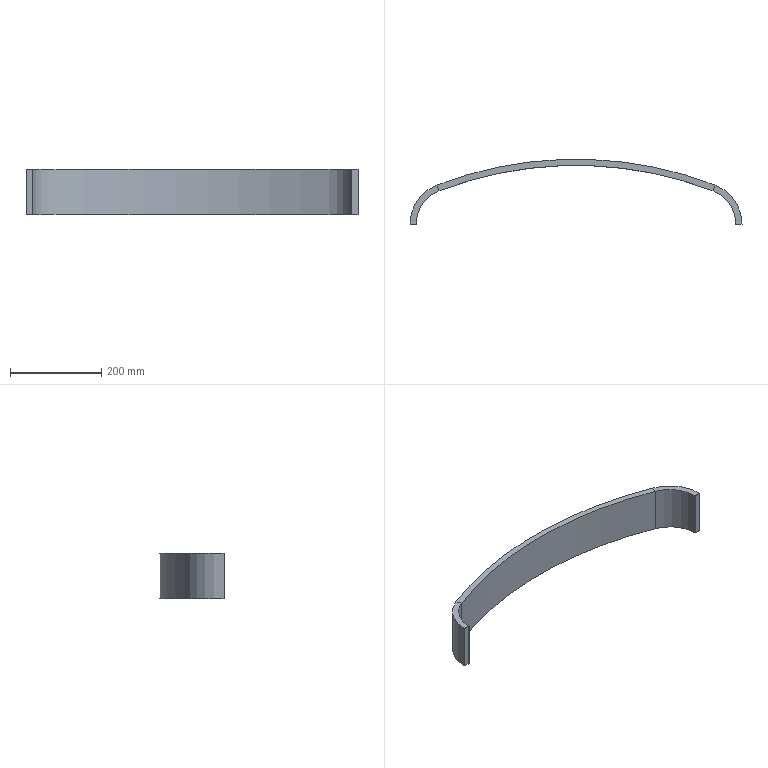Part | SolidWorks | features FlatPattern 1, HoleWzd 1, ICE 1, SMBaseFlange 1, SheetMetal 1 | 1 solid | 22 faces | box 727 x 142.5 x 100 mm | volume 1111821 mm3 | plane 16 | cylinder 6 | commonest cylinder face diameters 156.075 x2 183.075 x2 1670 x1 1697 x1
STEP:
#1=CARTESIAN_POINT('',(50.,0.4197,100.));
#2=VERTEX_POINT('',#1);
#3=CARTESIAN_POINT('',(36.5,0.4197,100.));
#4=VERTEX_POINT('',#3);
#5=CARTESIAN_POINT('',(50.,0.4197,100.));
#6=DIRECTION('',(-1.,0.,0.));
#7=VECTOR('',#6,1000.);
#8=LINE('',#5,#7);
#9=EDGE_CURVE('',#2,#4,#8,.T.);
#10=ORIENTED_EDGE('',*,*,#9,.F.);
#11=CARTESIAN_POINT('',(100.,73.246,100.));
#12=VERTEX_POINT('',#11);
#13=CARTESIAN_POINT('',(128.037,0.4197,100.));
#14=DIRECTION('',(0.,0.,1.));
#15=DIRECTION('',(1.,0.,0.));
#16=AXIS2_PLACEMENT_3D('',#13,#14,#15);
#17=CIRCLE('',#16,78.037);
#18=EDGE_CURVE('',#12,#2,#17,.T.);
#19=ORIENTED_EDGE('',*,*,#18,.F.);
#20=CARTESIAN_POINT('',(95.15,85.845,100.));
#21=VERTEX_POINT('',#20);
#22=CARTESIAN_POINT('',(100.,73.246,100.));
#23=DIRECTION('',(-0.3593,0.9332,0.));
#24=VECTOR('',#23,1000.);
#25=LINE('',#22,#24);
#26=EDGE_CURVE('',#12,#21,#25,.T.);
#27=ORIENTED_EDGE('',*,*,#26,.T.);
#28=CARTESIAN_POINT('',(128.037,0.4197,100.));
#29=DIRECTION('',(0.,0.,1.));
#30=DIRECTION('',(1.,0.,0.));
#31=AXIS2_PLACEMENT_3D('',#28,#29,#30);
#32=CIRCLE('',#31,91.537);
#33=EDGE_CURVE('',#21,#4,#32,.T.);
#34=ORIENTED_EDGE('',*,*,#33,.T.);
#35=EDGE_LOOP('',(#10,#19,#27,#34));
#36=FACE_OUTER_BOUND('',#35,.T.);
#37=CARTESIAN_POINT('',(50.,0.4197,100.));
#38=DIRECTION('',(0.,0.,1.));
#39=DIRECTION('',(1.,0.,0.));
#40=AXIS2_PLACEMENT_3D('',#37,#38,#39);
#41=PLANE('',#40);
#42=ADVANCED_FACE('',(#36),#41,.T.);
#43=CARTESIAN_POINT('',(36.5,0.4197,0.));
#44=VERTEX_POINT('',#43);
#45=CARTESIAN_POINT('',(50.,0.4197,0.));
#46=VERTEX_POINT('',#45);
#47=CARTESIAN_POINT('',(36.5,0.4197,0.));
#48=DIRECTION('',(1.,0.,0.));
#49=VECTOR('',#48,1000.);
#50=LINE('',#47,#49);
#51=EDGE_CURVE('',#44,#46,#50,.T.);
#52=ORIENTED_EDGE('',*,*,#51,.F.);
#53=CARTESIAN_POINT('',(95.15,85.845,0.));
#54=VERTEX_POINT('',#53);
#55=CARTESIAN_POINT('',(128.037,0.4197,0.));
#56=DIRECTION('',(0.,0.,1.));
#57=DIRECTION('',(1.,0.,0.));
#58=AXIS2_PLACEMENT_3D('',#55,#56,#57);
#59=CIRCLE('',#58,91.537);
#60=EDGE_CURVE('',#54,#44,#59,.T.);
#61=ORIENTED_EDGE('',*,*,#60,.F.);
#62=CARTESIAN_POINT('',(100.,73.246,0.));
#63=VERTEX_POINT('',#62);
#64=CARTESIAN_POINT('',(95.15,85.845,0.));
#65=DIRECTION('',(0.3593,-0.9332,0.));
#66=VECTOR('',#65,1000.);
#67=LINE('',#64,#66);
#68=EDGE_CURVE('',#54,#63,#67,.T.);
#69=ORIENTED_EDGE('',*,*,#68,.T.);
#70=CARTESIAN_POINT('',(128.037,0.4197,0.));
#71=DIRECTION('',(0.,0.,1.));
#72=DIRECTION('',(1.,0.,0.));
#73=AXIS2_PLACEMENT_3D('',#70,#71,#72);
#74=CIRCLE('',#73,78.037);
#75=EDGE_CURVE('',#63,#46,#74,.T.);
#76=ORIENTED_EDGE('',*,*,#75,.T.);
#77=EDGE_LOOP('',(#52,#61,#69,#76));
#78=FACE_OUTER_BOUND('',#77,.T.);
#79=CARTESIAN_POINT('',(36.5,0.4197,0.));
#80=DIRECTION('',(0.,0.,-1.));
#81=DIRECTION('',(-1.,0.,0.));
#82=AXIS2_PLACEMENT_3D('',#79,#80,#81);
#83=PLANE('',#82);
#84=ADVANCED_FACE('',(#78),#83,.T.);
#85=ORIENTED_EDGE('',*,*,#26,.F.);
#86=CARTESIAN_POINT('',(700.,73.246,100.));
#87=VERTEX_POINT('',#86);
#88=CARTESIAN_POINT('',(400.,-706.,100.));
#89=DIRECTION('',(0.,0.,1.));
#90=DIRECTION('',(-1.,0.,0.));
#91=AXIS2_PLACEMENT_3D('',#88,#89,#90);
#92=CIRCLE('',#91,835.);
#93=EDGE_CURVE('',#87,#12,#92,.T.);
#94=ORIENTED_EDGE('',*,*,#93,.F.);
#95=CARTESIAN_POINT('',(704.85,85.845,100.));
#96=VERTEX_POINT('',#95);
#97=CARTESIAN_POINT('',(700.,73.246,100.));
#98=DIRECTION('',(0.3593,0.9332,0.));
#99=VECTOR('',#98,1000.);
#100=LINE('',#97,#99);
#101=EDGE_CURVE('',#87,#96,#100,.T.);
#102=ORIENTED_EDGE('',*,*,#101,.T.);
#103=CARTESIAN_POINT('',(400.,-706.,100.));
#104=DIRECTION('',(0.,0.,1.));
#105=DIRECTION('',(1.,0.,0.));
#106=AXIS2_PLACEMENT_3D('',#103,#104,#105);
#107=CIRCLE('',#106,848.5);
#108=EDGE_CURVE('',#96,#21,#107,.T.);
#109=ORIENTED_EDGE('',*,*,#108,.T.);
#110=EDGE_LOOP('',(#85,#94,#102,#109));
#111=FACE_OUTER_BOUND('',#110,.T.);
#112=CARTESIAN_POINT('',(100.,73.246,100.));
#113=DIRECTION('',(0.,0.,1.));
#114=DIRECTION('',(1.,0.,0.));
#115=AXIS2_PLACEMENT_3D('',#112,#113,#114);
#116=PLANE('',#115);
#117=ADVANCED_FACE('',(#111),#116,.T.);
#118=ORIENTED_EDGE('',*,*,#68,.F.);
#119=CARTESIAN_POINT('',(704.85,85.845,0.));
#120=VERTEX_POINT('',#119);
#121=CARTESIAN_POINT('',(400.,-706.,0.));
#122=DIRECTION('',(0.,0.,1.));
#123=DIRECTION('',(1.,0.,0.));
#124=AXIS2_PLACEMENT_3D('',#121,#122,#123);
#125=CIRCLE('',#124,848.5);
#126=EDGE_CURVE('',#120,#54,#125,.T.);
#127=ORIENTED_EDGE('',*,*,#126,.F.);
#128=CARTESIAN_POINT('',(700.,73.246,0.));
#129=VERTEX_POINT('',#128);
#130=CARTESIAN_POINT('',(704.85,85.845,0.));
#131=DIRECTION('',(-0.3593,-0.9332,0.));
#132=VECTOR('',#131,1000.);
#133=LINE('',#130,#132);
#134=EDGE_CURVE('',#120,#129,#133,.T.);
#135=ORIENTED_EDGE('',*,*,#134,.T.);
#136=CARTESIAN_POINT('',(400.,-706.,0.));
#137=DIRECTION('',(0.,0.,1.));
#138=DIRECTION('',(-1.,0.,0.));
#139=AXIS2_PLACEMENT_3D('',#136,#137,#138);
#140=CIRCLE('',#139,835.);
#141=EDGE_CURVE('',#129,#63,#140,.T.);
#142=ORIENTED_EDGE('',*,*,#141,.T.);
#143=EDGE_LOOP('',(#118,#127,#135,#142));
#144=FACE_OUTER_BOUND('',#143,.T.);
#145=CARTESIAN_POINT('',(95.15,85.845,0.));
#146=DIRECTION('',(0.,0.,-1.));
#147=DIRECTION('',(-1.,0.,0.));
#148=AXIS2_PLACEMENT_3D('',#145,#146,#147);
#149=PLANE('',#148);
#150=ADVANCED_FACE('',(#144),#149,.T.);
#151=ORIENTED_EDGE('',*,*,#101,.F.);
#152=CARTESIAN_POINT('',(750.,0.4197,100.));
#153=VERTEX_POINT('',#152);
#154=CARTESIAN_POINT('',(671.963,0.4197,100.));
#155=DIRECTION('',(0.,0.,1.));
#156=DIRECTION('',(-1.,0.,0.));
#157=AXIS2_PLACEMENT_3D('',#154,#155,#156);
#158=CIRCLE('',#157,78.037);
#159=EDGE_CURVE('',#153,#87,#158,.T.);
#160=ORIENTED_EDGE('',*,*,#159,.F.);
#161=CARTESIAN_POINT('',(763.5,0.4197,100.));
#162=VERTEX_POINT('',#161);
#163=CARTESIAN_POINT('',(763.5,0.4197,100.));
#164=DIRECTION('',(-1.,0.,0.));
#165=VECTOR('',#164,1000.);
#166=LINE('',#163,#165);
#167=EDGE_CURVE('',#162,#153,#166,.T.);
#168=ORIENTED_EDGE('',*,*,#167,.F.);
#169=CARTESIAN_POINT('',(671.963,0.4197,100.));
#170=DIRECTION('',(0.,0.,1.));
#171=DIRECTION('',(1.,0.,0.));
#172=AXIS2_PLACEMENT_3D('',#169,#170,#171);
#173=CIRCLE('',#172,91.537);
#174=EDGE_CURVE('',#162,#96,#173,.T.);
#175=ORIENTED_EDGE('',*,*,#174,.T.);
#176=EDGE_LOOP('',(#151,#160,#168,#175));
#177=FACE_OUTER_BOUND('',#176,.T.);
#178=CARTESIAN_POINT('',(700.,73.246,100.));
#179=DIRECTION('',(0.,0.,1.));
#180=DIRECTION('',(1.,0.,0.));
#181=AXIS2_PLACEMENT_3D('',#178,#179,#180);
#182=PLANE('',#181);
#183=ADVANCED_FACE('',(#177),#182,.T.);
#184=CARTESIAN_POINT('',(50.,0.,100.));
#185=VERTEX_POINT('',#184);
#186=CARTESIAN_POINT('',(50.,0.,100.));
#187=DIRECTION('',(0.,-1.,0.));
#188=VECTOR('',#187,1000.);
#189=LINE('',#186,#188);
#190=EDGE_CURVE('',#2,#185,#189,.T.);
#191=ORIENTED_EDGE('',*,*,#190,.F.);
#192=ORIENTED_EDGE('',*,*,#9,.T.);
#193=CARTESIAN_POINT('',(36.5,0.,100.));
#194=VERTEX_POINT('',#193);
#195=CARTESIAN_POINT('',(36.5,0.,100.));
#196=DIRECTION('',(0.,-1.,0.));
#197=VECTOR('',#196,1000.);
#198=LINE('',#195,#197);
#199=EDGE_CURVE('',#4,#194,#198,.T.);
#200=ORIENTED_EDGE('',*,*,#199,.T.);
#201=CARTESIAN_POINT('',(50.,0.,100.));
#202=DIRECTION('',(-1.,0.,0.));
#203=VECTOR('',#202,1000.);
#204=LINE('',#201,#203);
#205=EDGE_CURVE('',#185,#194,#204,.T.);
#206=ORIENTED_EDGE('',*,*,#205,.F.);
#207=EDGE_LOOP('',(#191,#192,#200,#206));
#208=FACE_OUTER_BOUND('',#207,.T.);
#209=CARTESIAN_POINT('',(763.5,0.4197,100.));
#210=DIRECTION('',(0.,0.,1.));
#211=DIRECTION('',(1.,0.,0.));
#212=AXIS2_PLACEMENT_3D('',#209,#210,#211);
#213=PLANE('',#212);
#214=ADVANCED_FACE('',(#208),#213,.T.);
#215=CARTESIAN_POINT('',(750.,0.4197,0.));
#216=VERTEX_POINT('',#215);
#217=CARTESIAN_POINT('',(763.5,0.4197,0.));
#218=VERTEX_POINT('',#217);
#219=CARTESIAN_POINT('',(750.,0.4197,0.));
#220=DIRECTION('',(1.,0.,0.));
#221=VECTOR('',#220,1000.);
#222=LINE('',#219,#221);
#223=EDGE_CURVE('',#216,#218,#222,.T.);
#224=ORIENTED_EDGE('',*,*,#223,.F.);
#225=CARTESIAN_POINT('',(671.963,0.4197,0.));
#226=DIRECTION('',(0.,0.,1.));
#227=DIRECTION('',(-1.,0.,0.));
#228=AXIS2_PLACEMENT_3D('',#225,#226,#227);
#229=CIRCLE('',#228,78.037);
#230=EDGE_CURVE('',#216,#129,#229,.T.);
#231=ORIENTED_EDGE('',*,*,#230,.T.);
#232=ORIENTED_EDGE('',*,*,#134,.F.);
#233=CARTESIAN_POINT('',(671.963,0.4197,0.));
#234=DIRECTION('',(0.,0.,1.));
#235=DIRECTION('',(1.,0.,0.));
#236=AXIS2_PLACEMENT_3D('',#233,#234,#235);
#237=CIRCLE('',#236,91.537);
#238=EDGE_CURVE('',#218,#120,#237,.T.);
#239=ORIENTED_EDGE('',*,*,#238,.F.);
#240=EDGE_LOOP('',(#224,#231,#232,#239));
#241=FACE_OUTER_BOUND('',#240,.T.);
#242=CARTESIAN_POINT('',(750.,0.4197,0.));
#243=DIRECTION('',(0.,0.,-1.));
#244=DIRECTION('',(-1.,0.,0.));
#245=AXIS2_PLACEMENT_3D('',#242,#243,#244);
#246=PLANE('',#245);
#247=ADVANCED_FACE('',(#241),#246,.T.);
#248=CARTESIAN_POINT('',(750.,0.,0.));
#249=VERTEX_POINT('',#248);
#250=CARTESIAN_POINT('',(750.,0.,0.));
#251=DIRECTION('',(0.,1.,0.));
#252=VECTOR('',#251,1000.);
#253=LINE('',#250,#252);
#254=EDGE_CURVE('',#249,#216,#253,.T.);
#255=ORIENTED_EDGE('',*,*,#254,.T.);
#256=ORIENTED_EDGE('',*,*,#223,.T.);
#257=CARTESIAN_POINT('',(763.5,0.,0.));
#258=VERTEX_POINT('',#257);
#259=CARTESIAN_POINT('',(763.5,0.,0.));
#260=DIRECTION('',(0.,1.,0.));
#261=VECTOR('',#260,1000.);
#262=LINE('',#259,#261);
#263=EDGE_CURVE('',#258,#218,#262,.T.);
#264=ORIENTED_EDGE('',*,*,#263,.F.);
#265=CARTESIAN_POINT('',(763.5,0.,0.));
#266=DIRECTION('',(-1.,0.,0.));
#267=VECTOR('',#266,1000.);
#268=LINE('',#265,#267);
#269=EDGE_CURVE('',#258,#249,#268,.T.);
#270=ORIENTED_EDGE('',*,*,#269,.T.);
#271=EDGE_LOOP('',(#255,#256,#264,#270));
#272=FACE_OUTER_BOUND('',#271,.T.);
#273=CARTESIAN_POINT('',(704.85,85.845,0.));
#274=DIRECTION('',(0.,0.,-1.));
#275=DIRECTION('',(-1.,0.,0.));
#276=AXIS2_PLACEMENT_3D('',#273,#274,#275);
#277=PLANE('',#276);
#278=ADVANCED_FACE('',(#272),#277,.T.);
#279=CARTESIAN_POINT('',(36.5,0.,0.));
#280=VERTEX_POINT('',#279);
#281=CARTESIAN_POINT('',(36.5,0.,0.));
#282=DIRECTION('',(0.,-1.,0.));
#283=VECTOR('',#282,1000.);
#284=LINE('',#281,#283);
#285=EDGE_CURVE('',#44,#280,#284,.T.);
#286=ORIENTED_EDGE('',*,*,#285,.T.);
#287=CARTESIAN_POINT('',(36.5,0.,100.));
#288=DIRECTION('',(0.,0.,-1.));
#289=VECTOR('',#288,1000.);
#290=LINE('',#287,#289);
#291=EDGE_CURVE('',#194,#280,#290,.T.);
#292=ORIENTED_EDGE('',*,*,#291,.F.);
#293=ORIENTED_EDGE('',*,*,#199,.F.);
#294=CARTESIAN_POINT('',(36.5,0.4197,100.));
#295=DIRECTION('',(0.,0.,-1.));
#296=VECTOR('',#295,1000.);
#297=LINE('',#294,#296);
#298=EDGE_CURVE('',#4,#44,#297,.T.);
#299=ORIENTED_EDGE('',*,*,#298,.T.);
#300=EDGE_LOOP('',(#286,#292,#293,#299));
#301=FACE_OUTER_BOUND('',#300,.T.);
#302=CARTESIAN_POINT('',(36.5,0.,100.));
#303=DIRECTION('',(1.,0.,0.));
#304=DIRECTION('',(0.,1.,0.));
#305=AXIS2_PLACEMENT_3D('',#302,#303,#304);
#306=PLANE('',#305);
#307=ADVANCED_FACE('',(#301),#306,.F.);
#308=CARTESIAN_POINT('',(50.,0.,0.));
#309=VERTEX_POINT('',#308);
#310=CARTESIAN_POINT('',(50.,0.,0.));
#311=DIRECTION('',(-1.,0.,0.));
#312=VECTOR('',#311,1000.);
#313=LINE('',#310,#312);
#314=EDGE_CURVE('',#309,#280,#313,.T.);
#315=ORIENTED_EDGE('',*,*,#314,.F.);
#316=CARTESIAN_POINT('',(50.,0.,100.));
#317=DIRECTION('',(0.,0.,-1.));
#318=VECTOR('',#317,1000.);
#319=LINE('',#316,#318);
#320=EDGE_CURVE('',#185,#309,#319,.T.);
#321=ORIENTED_EDGE('',*,*,#320,.F.);
#322=ORIENTED_EDGE('',*,*,#205,.T.);
#323=ORIENTED_EDGE('',*,*,#291,.T.);
#324=EDGE_LOOP('',(#315,#321,#322,#323));
#325=FACE_OUTER_BOUND('',#324,.T.);
#326=CARTESIAN_POINT('',(50.,0.,100.));
#327=DIRECTION('',(0.,-1.,0.));
#328=DIRECTION('',(1.,0.,0.));
#329=AXIS2_PLACEMENT_3D('',#326,#327,#328);
#330=PLANE('',#329);
#331=ADVANCED_FACE('',(#325),#330,.T.);
#332=CARTESIAN_POINT('',(50.,0.,0.));
#333=DIRECTION('',(0.,-1.,0.));
#334=VECTOR('',#333,1000.);
#335=LINE('',#332,#334);
#336=EDGE_CURVE('',#46,#309,#335,.T.);
#337=ORIENTED_EDGE('',*,*,#336,.F.);
#338=CARTESIAN_POINT('',(50.,0.4197,100.));
#339=DIRECTION('',(0.,0.,-1.));
#340=VECTOR('',#339,1000.);
#341=LINE('',#338,#340);
#342=EDGE_CURVE('',#2,#46,#341,.T.);
#343=ORIENTED_EDGE('',*,*,#342,.F.);
#344=ORIENTED_EDGE('',*,*,#190,.T.);
#345=ORIENTED_EDGE('',*,*,#320,.T.);
#346=EDGE_LOOP('',(#337,#343,#344,#345));
#347=FACE_OUTER_BOUND('',#346,.T.);
#348=CARTESIAN_POINT('',(50.,0.,100.));
#349=DIRECTION('',(1.,0.,0.));
#350=DIRECTION('',(0.,1.,0.));
#351=AXIS2_PLACEMENT_3D('',#348,#349,#350);
#352=PLANE('',#351);
#353=ADVANCED_FACE('',(#347),#352,.T.);
#354=ORIENTED_EDGE('',*,*,#75,.F.);
#355=CARTESIAN_POINT('',(100.,73.246,100.));
#356=DIRECTION('',(0.,0.,-1.));
#357=VECTOR('',#356,1000.);
#358=LINE('',#355,#357);
#359=EDGE_CURVE('',#12,#63,#358,.T.);
#360=ORIENTED_EDGE('',*,*,#359,.F.);
#361=ORIENTED_EDGE('',*,*,#18,.T.);
#362=ORIENTED_EDGE('',*,*,#342,.T.);
#363=EDGE_LOOP('',(#354,#360,#361,#362));
#364=FACE_OUTER_BOUND('',#363,.T.);
#365=CARTESIAN_POINT('',(128.037,0.4197,100.));
#366=DIRECTION('',(0.,0.,-1.));
#367=DIRECTION('',(-1.,0.,0.));
#368=AXIS2_PLACEMENT_3D('',#365,#366,#367);
#369=CYLINDRICAL_SURFACE('',#368,78.037);
#370=ADVANCED_FACE('',(#364),#369,.F.);
#371=ORIENTED_EDGE('',*,*,#141,.F.);
#372=CARTESIAN_POINT('',(700.,73.246,100.));
#373=DIRECTION('',(0.,0.,-1.));
#374=VECTOR('',#373,1000.);
#375=LINE('',#372,#374);
#376=EDGE_CURVE('',#87,#129,#375,.T.);
#377=ORIENTED_EDGE('',*,*,#376,.F.);
#378=ORIENTED_EDGE('',*,*,#93,.T.);
#379=ORIENTED_EDGE('',*,*,#359,.T.);
#380=EDGE_LOOP('',(#371,#377,#378,#379));
#381=FACE_OUTER_BOUND('',#380,.T.);
#382=CARTESIAN_POINT('',(400.,-706.,100.));
#383=DIRECTION('',(0.,0.,-1.));
#384=DIRECTION('',(-1.,0.,0.));
#385=AXIS2_PLACEMENT_3D('',#382,#383,#384);
#386=CYLINDRICAL_SURFACE('',#385,835.);
#387=ADVANCED_FACE('',(#381),#386,.F.);
#388=ORIENTED_EDGE('',*,*,#230,.F.);
#389=CARTESIAN_POINT('',(750.,0.4197,100.));
#390=DIRECTION('',(0.,0.,-1.));
#391=VECTOR('',#390,1000.);
#392=LINE('',#389,#391);
#393=EDGE_CURVE('',#153,#216,#392,.T.);
#394=ORIENTED_EDGE('',*,*,#393,.F.);
#395=ORIENTED_EDGE('',*,*,#159,.T.);
#396=ORIENTED_EDGE('',*,*,#376,.T.);
#397=EDGE_LOOP('',(#388,#394,#395,#396));
#398=FACE_OUTER_BOUND('',#397,.T.);
#399=CARTESIAN_POINT('',(671.963,0.4197,100.));
#400=DIRECTION('',(0.,0.,-1.));
#401=DIRECTION('',(-1.,0.,0.));
#402=AXIS2_PLACEMENT_3D('',#399,#400,#401);
#403=CYLINDRICAL_SURFACE('',#402,78.037);
#404=ADVANCED_FACE('',(#398),#403,.F.);
#405=ORIENTED_EDGE('',*,*,#254,.F.);
#406=CARTESIAN_POINT('',(750.,0.,100.));
#407=VERTEX_POINT('',#406);
#408=CARTESIAN_POINT('',(750.,0.,100.));
#409=DIRECTION('',(0.,0.,-1.));
#410=VECTOR('',#409,1000.);
#411=LINE('',#408,#410);
#412=EDGE_CURVE('',#407,#249,#411,.T.);
#413=ORIENTED_EDGE('',*,*,#412,.F.);
#414=CARTESIAN_POINT('',(750.,0.,100.));
#415=DIRECTION('',(0.,1.,0.));
#416=VECTOR('',#415,1000.);
#417=LINE('',#414,#416);
#418=EDGE_CURVE('',#407,#153,#417,.T.);
#419=ORIENTED_EDGE('',*,*,#418,.T.);
#420=ORIENTED_EDGE('',*,*,#393,.T.);
#421=EDGE_LOOP('',(#405,#413,#419,#420));
#422=FACE_OUTER_BOUND('',#421,.T.);
#423=CARTESIAN_POINT('',(750.,0.,100.));
#424=DIRECTION('',(-1.,0.,0.));
#425=DIRECTION('',(0.,0.,1.));
#426=AXIS2_PLACEMENT_3D('',#423,#424,#425);
#427=PLANE('',#426);
#428=ADVANCED_FACE('',(#422),#427,.T.);
#429=ORIENTED_EDGE('',*,*,#269,.F.);
#430=CARTESIAN_POINT('',(763.5,0.,100.));
#431=VERTEX_POINT('',#430);
#432=CARTESIAN_POINT('',(763.5,0.,100.));
#433=DIRECTION('',(0.,0.,-1.));
#434=VECTOR('',#433,1000.);
#435=LINE('',#432,#434);
#436=EDGE_CURVE('',#431,#258,#435,.T.);
#437=ORIENTED_EDGE('',*,*,#436,.F.);
#438=CARTESIAN_POINT('',(763.5,0.,100.));
#439=DIRECTION('',(-1.,0.,0.));
#440=VECTOR('',#439,1000.);
#441=LINE('',#438,#440);
#442=EDGE_CURVE('',#431,#407,#441,.T.);
#443=ORIENTED_EDGE('',*,*,#442,.T.);
#444=ORIENTED_EDGE('',*,*,#412,.T.);
#445=EDGE_LOOP('',(#429,#437,#443,#444));
#446=FACE_OUTER_BOUND('',#445,.T.);
#447=CARTESIAN_POINT('',(763.5,0.,100.));
#448=DIRECTION('',(0.,-1.,0.));
#449=DIRECTION('',(0.,0.,-1.));
#450=AXIS2_PLACEMENT_3D('',#447,#448,#449);
#451=PLANE('',#450);
#452=ADVANCED_FACE('',(#446),#451,.T.);
#453=ORIENTED_EDGE('',*,*,#263,.T.);
#454=CARTESIAN_POINT('',(763.5,0.4197,100.));
#455=DIRECTION('',(0.,0.,-1.));
#456=VECTOR('',#455,1000.);
#457=LINE('',#454,#456);
#458=EDGE_CURVE('',#162,#218,#457,.T.);
#459=ORIENTED_EDGE('',*,*,#458,.F.);
#460=CARTESIAN_POINT('',(763.5,0.,100.));
#461=DIRECTION('',(0.,1.,0.));
#462=VECTOR('',#461,1000.);
#463=LINE('',#460,#462);
#464=EDGE_CURVE('',#431,#162,#463,.T.);
#465=ORIENTED_EDGE('',*,*,#464,.F.);
#466=ORIENTED_EDGE('',*,*,#436,.T.);
#467=EDGE_LOOP('',(#453,#459,#465,#466));
#468=FACE_OUTER_BOUND('',#467,.T.);
#469=CARTESIAN_POINT('',(763.5,0.,100.));
#470=DIRECTION('',(-1.,0.,0.));
#471=DIRECTION('',(0.,0.,1.));
#472=AXIS2_PLACEMENT_3D('',#469,#470,#471);
#473=PLANE('',#472);
#474=ADVANCED_FACE('',(#468),#473,.F.);
#475=ORIENTED_EDGE('',*,*,#238,.T.);
#476=CARTESIAN_POINT('',(704.85,85.845,100.));
#477=DIRECTION('',(0.,0.,-1.));
#478=VECTOR('',#477,1000.);
#479=LINE('',#476,#478);
#480=EDGE_CURVE('',#96,#120,#479,.T.);
#481=ORIENTED_EDGE('',*,*,#480,.F.);
#482=ORIENTED_EDGE('',*,*,#174,.F.);
#483=ORIENTED_EDGE('',*,*,#458,.T.);
#484=EDGE_LOOP('',(#475,#481,#482,#483));
#485=FACE_OUTER_BOUND('',#484,.T.);
#486=CARTESIAN_POINT('',(671.963,0.4197,100.));
#487=DIRECTION('',(0.,0.,-1.));
#488=DIRECTION('',(-1.,0.,0.));
#489=AXIS2_PLACEMENT_3D('',#486,#487,#488);
#490=CYLINDRICAL_SURFACE('',#489,91.537);
#491=ADVANCED_FACE('',(#485),#490,.T.);
#492=ORIENTED_EDGE('',*,*,#126,.T.);
#493=CARTESIAN_POINT('',(95.15,85.845,100.));
#494=DIRECTION('',(0.,0.,-1.));
#495=VECTOR('',#494,1000.);
#496=LINE('',#493,#495);
#497=EDGE_CURVE('',#21,#54,#496,.T.);
#498=ORIENTED_EDGE('',*,*,#497,.F.);
#499=ORIENTED_EDGE('',*,*,#108,.F.);
#500=ORIENTED_EDGE('',*,*,#480,.T.);
#501=EDGE_LOOP('',(#492,#498,#499,#500));
#502=FACE_OUTER_BOUND('',#501,.T.);
#503=CARTESIAN_POINT('',(400.,-706.,100.));
#504=DIRECTION('',(0.,0.,-1.));
#505=DIRECTION('',(-1.,0.,0.));
#506=AXIS2_PLACEMENT_3D('',#503,#504,#505);
#507=CYLINDRICAL_SURFACE('',#506,848.5);
#508=ADVANCED_FACE('',(#502),#507,.T.);
#509=ORIENTED_EDGE('',*,*,#60,.T.);
#510=ORIENTED_EDGE('',*,*,#298,.F.);
#511=ORIENTED_EDGE('',*,*,#33,.F.);
#512=ORIENTED_EDGE('',*,*,#497,.T.);
#513=EDGE_LOOP('',(#509,#510,#511,#512));
#514=FACE_OUTER_BOUND('',#513,.T.);
#515=CARTESIAN_POINT('',(128.037,0.4197,100.));
#516=DIRECTION('',(0.,0.,-1.));
#517=DIRECTION('',(-1.,0.,0.));
#518=AXIS2_PLACEMENT_3D('',#515,#516,#517);
#519=CYLINDRICAL_SURFACE('',#518,91.537);
#520=ADVANCED_FACE('',(#514),#519,.T.);
#521=ORIENTED_EDGE('',*,*,#464,.T.);
#522=ORIENTED_EDGE('',*,*,#167,.T.);
#523=ORIENTED_EDGE('',*,*,#418,.F.);
#524=ORIENTED_EDGE('',*,*,#442,.F.);
#525=EDGE_LOOP('',(#521,#522,#523,#524));
#526=FACE_OUTER_BOUND('',#525,.T.);
#527=CARTESIAN_POINT('',(128.037,0.4197,100.));
#528=DIRECTION('',(0.,0.,1.));
#529=DIRECTION('',(1.,0.,0.));
#530=AXIS2_PLACEMENT_3D('',#527,#528,#529);
#531=PLANE('',#530);
#532=ADVANCED_FACE('',(#526),#531,.T.);
#533=ORIENTED_EDGE('',*,*,#285,.F.);
#534=ORIENTED_EDGE('',*,*,#51,.T.);
#535=ORIENTED_EDGE('',*,*,#336,.T.);
#536=ORIENTED_EDGE('',*,*,#314,.T.);
#537=EDGE_LOOP('',(#533,#534,#535,#536));
#538=FACE_OUTER_BOUND('',#537,.T.);
#539=CARTESIAN_POINT('',(128.037,0.4197,0.));
#540=DIRECTION('',(0.,0.,1.));
#541=DIRECTION('',(1.,0.,0.));
#542=AXIS2_PLACEMENT_3D('',#539,#540,#541);
#543=PLANE('',#542);
#544=ADVANCED_FACE('',(#538),#543,.F.);
#545=CLOSED_SHELL('',(#42,#84,#117,#150,#183,#214,#247,#278,#307,#331,#353,#370,#387,#404,#428,#452,#474,#491,#508,#520,#532,#544));
#546=MANIFOLD_SOLID_BREP('',#545);
#547=CARTESIAN_POINT('',(0.,0.,0.));
#548=DIRECTION('',(0.,0.,1.));
#549=DIRECTION('',(1.,0.,0.));
#550=AXIS2_PLACEMENT_3D('',#547,#548,#549);
#551=(LENGTH_UNIT()NAMED_UNIT(*)SI_UNIT(.MILLI.,.METRE.));
#552=UNCERTAINTY_MEASURE_WITH_UNIT(LENGTH_MEASURE(0.00001),#551,'','');
#553=(NAMED_UNIT(*)PLANE_ANGLE_UNIT()SI_UNIT($,.RADIAN.));
#554=(NAMED_UNIT(*)SI_UNIT($,.STERADIAN.)SOLID_ANGLE_UNIT());
#555=(GEOMETRIC_REPRESENTATION_CONTEXT(3)GLOBAL_UNCERTAINTY_ASSIGNED_CONTEXT((#552))GLOBAL_UNIT_ASSIGNED_CONTEXT((#551,#553,#554))REPRESENTATION_CONTEXT('',''));
#556=ADVANCED_BREP_SHAPE_REPRESENTATION('',(#546,#550),#555);